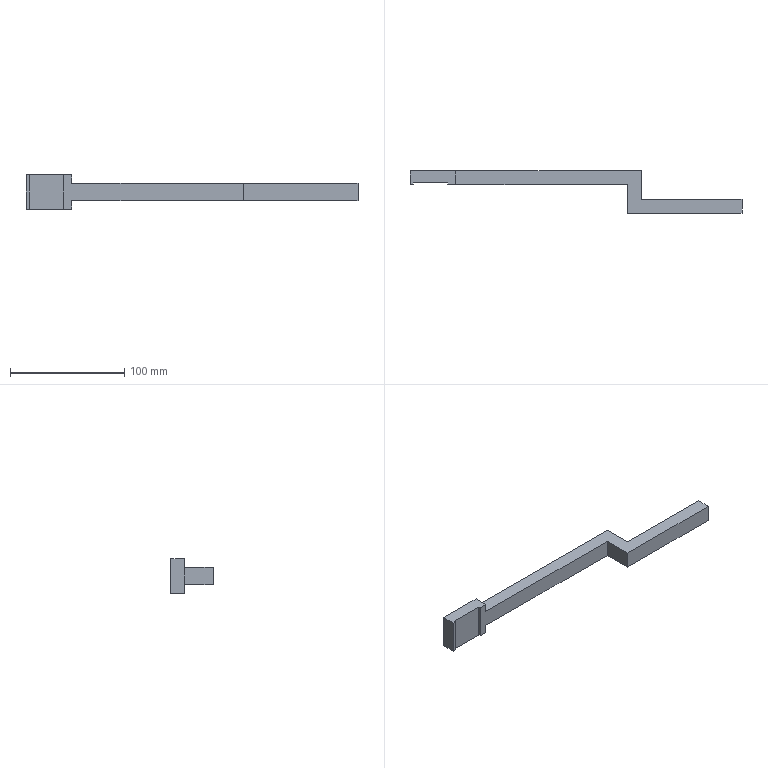Part | SolidWorks | features ICE 2, Extrusion 1 | 1 solid | 18 faces | box 290 x 37 x 30 mm | volume 62550 mm3 | plane 18
STEP:
#1=CARTESIAN_POINT('',(-37.,-12.,-15.));
#2=VERTEX_POINT('',#1);
#3=CARTESIAN_POINT('',(-37.,-12.,15.));
#4=VERTEX_POINT('',#3);
#5=CARTESIAN_POINT('',(-37.,-12.,-15.));
#6=DIRECTION('',(0.,0.,1.));
#7=VECTOR('',#6,1000.);
#8=LINE('',#5,#7);
#9=EDGE_CURVE('',#2,#4,#8,.T.);
#10=ORIENTED_EDGE('',*,*,#9,.T.);
#11=CARTESIAN_POINT('',(-40.,-12.,15.));
#12=VERTEX_POINT('',#11);
#13=CARTESIAN_POINT('',(0.,-12.,15.));
#14=DIRECTION('',(-1.,0.,0.));
#15=VECTOR('',#14,1000.);
#16=LINE('',#13,#15);
#17=EDGE_CURVE('',#4,#12,#16,.T.);
#18=ORIENTED_EDGE('',*,*,#17,.T.);
#19=CARTESIAN_POINT('',(-40.,-12.,-15.));
#20=VERTEX_POINT('',#19);
#21=CARTESIAN_POINT('',(-40.,-12.,15.));
#22=DIRECTION('',(0.,0.,-1.));
#23=VECTOR('',#22,1000.);
#24=LINE('',#21,#23);
#25=EDGE_CURVE('',#12,#20,#24,.T.);
#26=ORIENTED_EDGE('',*,*,#25,.T.);
#27=CARTESIAN_POINT('',(0.,-12.,-15.));
#28=DIRECTION('',(1.,0.,0.));
#29=VECTOR('',#28,1000.);
#30=LINE('',#27,#29);
#31=EDGE_CURVE('',#20,#2,#30,.T.);
#32=ORIENTED_EDGE('',*,*,#31,.T.);
#33=EDGE_LOOP('',(#10,#18,#26,#32));
#34=FACE_OUTER_BOUND('',#33,.T.);
#35=CARTESIAN_POINT('',(150.,-12.,7.5));
#36=DIRECTION('',(0.,1.,0.));
#37=DIRECTION('',(-1.,0.,0.));
#38=AXIS2_PLACEMENT_3D('',#35,#36,#37);
#39=PLANE('',#38);
#40=ADVANCED_FACE('',(#34),#39,.F.);
#41=CARTESIAN_POINT('',(-7.,-12.,15.));
#42=VERTEX_POINT('',#41);
#43=CARTESIAN_POINT('',(-7.,-12.,-15.));
#44=VERTEX_POINT('',#43);
#45=CARTESIAN_POINT('',(-7.,-12.,-15.));
#46=DIRECTION('',(0.,0.,-1.));
#47=VECTOR('',#46,1000.);
#48=LINE('',#45,#47);
#49=EDGE_CURVE('',#42,#44,#48,.T.);
#50=ORIENTED_EDGE('',*,*,#49,.T.);
#51=CARTESIAN_POINT('',(0.,-12.,-15.));
#52=VERTEX_POINT('',#51);
#53=CARTESIAN_POINT('',(0.,-12.,-15.));
#54=DIRECTION('',(1.,0.,0.));
#55=VECTOR('',#54,1000.);
#56=LINE('',#53,#55);
#57=EDGE_CURVE('',#44,#52,#56,.T.);
#58=ORIENTED_EDGE('',*,*,#57,.T.);
#59=CARTESIAN_POINT('',(0.,-12.,-7.5));
#60=VERTEX_POINT('',#59);
#61=CARTESIAN_POINT('',(0.,-12.,15.));
#62=DIRECTION('',(0.,0.,1.));
#63=VECTOR('',#62,1000.);
#64=LINE('',#61,#63);
#65=EDGE_CURVE('',#52,#60,#64,.T.);
#66=ORIENTED_EDGE('',*,*,#65,.T.);
#67=CARTESIAN_POINT('',(150.,-12.,-7.5));
#68=VERTEX_POINT('',#67);
#69=CARTESIAN_POINT('',(150.,-12.,-7.5));
#70=DIRECTION('',(1.,0.,0.));
#71=VECTOR('',#70,1000.);
#72=LINE('',#69,#71);
#73=EDGE_CURVE('',#60,#68,#72,.T.);
#74=ORIENTED_EDGE('',*,*,#73,.T.);
#75=CARTESIAN_POINT('',(150.,-12.,7.5));
#76=VERTEX_POINT('',#75);
#77=CARTESIAN_POINT('',(150.,-12.,7.5));
#78=DIRECTION('',(0.,0.,-1.));
#79=VECTOR('',#78,1000.);
#80=LINE('',#77,#79);
#81=EDGE_CURVE('',#76,#68,#80,.T.);
#82=ORIENTED_EDGE('',*,*,#81,.F.);
#83=CARTESIAN_POINT('',(0.,-12.,7.5));
#84=VERTEX_POINT('',#83);
#85=CARTESIAN_POINT('',(150.,-12.,7.5));
#86=DIRECTION('',(1.,0.,0.));
#87=VECTOR('',#86,1000.);
#88=LINE('',#85,#87);
#89=EDGE_CURVE('',#84,#76,#88,.T.);
#90=ORIENTED_EDGE('',*,*,#89,.F.);
#91=CARTESIAN_POINT('',(0.,-12.,15.));
#92=VERTEX_POINT('',#91);
#93=CARTESIAN_POINT('',(0.,-12.,15.));
#94=DIRECTION('',(0.,0.,1.));
#95=VECTOR('',#94,1000.);
#96=LINE('',#93,#95);
#97=EDGE_CURVE('',#84,#92,#96,.T.);
#98=ORIENTED_EDGE('',*,*,#97,.T.);
#99=CARTESIAN_POINT('',(0.,-12.,15.));
#100=DIRECTION('',(-1.,0.,0.));
#101=VECTOR('',#100,1000.);
#102=LINE('',#99,#101);
#103=EDGE_CURVE('',#92,#42,#102,.T.);
#104=ORIENTED_EDGE('',*,*,#103,.T.);
#105=EDGE_LOOP('',(#50,#58,#66,#74,#82,#90,#98,#104));
#106=FACE_OUTER_BOUND('',#105,.T.);
#107=CARTESIAN_POINT('',(150.,-12.,7.5));
#108=DIRECTION('',(0.,1.,0.));
#109=DIRECTION('',(-1.,0.,0.));
#110=AXIS2_PLACEMENT_3D('',#107,#108,#109);
#111=PLANE('',#110);
#112=ADVANCED_FACE('',(#106),#111,.F.);
#113=CARTESIAN_POINT('',(-7.,-10.5,-15.));
#114=VERTEX_POINT('',#113);
#115=CARTESIAN_POINT('',(-37.,-10.5,-15.));
#116=VERTEX_POINT('',#115);
#117=CARTESIAN_POINT('',(-37.,-10.5,-15.));
#118=DIRECTION('',(-1.,0.,0.));
#119=VECTOR('',#118,1000.);
#120=LINE('',#117,#119);
#121=EDGE_CURVE('',#114,#116,#120,.T.);
#122=ORIENTED_EDGE('',*,*,#121,.T.);
#123=CARTESIAN_POINT('',(-37.,-10.5,-15.));
#124=DIRECTION('',(0.,-1.,0.));
#125=VECTOR('',#124,1000.);
#126=LINE('',#123,#125);
#127=EDGE_CURVE('',#116,#2,#126,.T.);
#128=ORIENTED_EDGE('',*,*,#127,.T.);
#129=ORIENTED_EDGE('',*,*,#31,.F.);
#130=CARTESIAN_POINT('',(-40.,0.,-15.));
#131=VERTEX_POINT('',#130);
#132=CARTESIAN_POINT('',(-40.,-62.,-15.));
#133=DIRECTION('',(0.,1.,0.));
#134=VECTOR('',#133,1000.);
#135=LINE('',#132,#134);
#136=EDGE_CURVE('',#20,#131,#135,.T.);
#137=ORIENTED_EDGE('',*,*,#136,.T.);
#138=CARTESIAN_POINT('',(0.,0.,-15.));
#139=VERTEX_POINT('',#138);
#140=CARTESIAN_POINT('',(0.,0.,-15.));
#141=DIRECTION('',(-1.,0.,0.));
#142=VECTOR('',#141,1000.);
#143=LINE('',#140,#142);
#144=EDGE_CURVE('',#139,#131,#143,.T.);
#145=ORIENTED_EDGE('',*,*,#144,.F.);
#146=CARTESIAN_POINT('',(0.,-62.,-15.));
#147=DIRECTION('',(0.,1.,0.));
#148=VECTOR('',#147,1000.);
#149=LINE('',#146,#148);
#150=EDGE_CURVE('',#52,#139,#149,.T.);
#151=ORIENTED_EDGE('',*,*,#150,.F.);
#152=ORIENTED_EDGE('',*,*,#57,.F.);
#153=CARTESIAN_POINT('',(-7.,-10.5,-15.));
#154=DIRECTION('',(0.,-1.,0.));
#155=VECTOR('',#154,1000.);
#156=LINE('',#153,#155);
#157=EDGE_CURVE('',#114,#44,#156,.T.);
#158=ORIENTED_EDGE('',*,*,#157,.F.);
#159=EDGE_LOOP('',(#122,#128,#129,#137,#145,#151,#152,#158));
#160=FACE_OUTER_BOUND('',#159,.T.);
#161=CARTESIAN_POINT('',(0.,-62.,-15.));
#162=DIRECTION('',(0.,0.,-1.));
#163=DIRECTION('',(-1.,0.,0.));
#164=AXIS2_PLACEMENT_3D('',#161,#162,#163);
#165=PLANE('',#164);
#166=ADVANCED_FACE('',(#160),#165,.T.);
#167=ORIENTED_EDGE('',*,*,#17,.F.);
#168=CARTESIAN_POINT('',(-37.,-10.5,15.));
#169=VERTEX_POINT('',#168);
#170=CARTESIAN_POINT('',(-37.,-10.5,15.));
#171=DIRECTION('',(0.,-1.,0.));
#172=VECTOR('',#171,1000.);
#173=LINE('',#170,#172);
#174=EDGE_CURVE('',#169,#4,#173,.T.);
#175=ORIENTED_EDGE('',*,*,#174,.F.);
#176=CARTESIAN_POINT('',(-7.,-10.5,15.));
#177=VERTEX_POINT('',#176);
#178=CARTESIAN_POINT('',(-37.,-10.5,15.));
#179=DIRECTION('',(1.,0.,0.));
#180=VECTOR('',#179,1000.);
#181=LINE('',#178,#180);
#182=EDGE_CURVE('',#169,#177,#181,.T.);
#183=ORIENTED_EDGE('',*,*,#182,.T.);
#184=CARTESIAN_POINT('',(-7.,-10.5,15.));
#185=DIRECTION('',(0.,-1.,0.));
#186=VECTOR('',#185,1000.);
#187=LINE('',#184,#186);
#188=EDGE_CURVE('',#177,#42,#187,.T.);
#189=ORIENTED_EDGE('',*,*,#188,.T.);
#190=ORIENTED_EDGE('',*,*,#103,.F.);
#191=CARTESIAN_POINT('',(0.,0.,15.));
#192=VERTEX_POINT('',#191);
#193=CARTESIAN_POINT('',(0.,-62.,15.));
#194=DIRECTION('',(0.,1.,0.));
#195=VECTOR('',#194,1000.);
#196=LINE('',#193,#195);
#197=EDGE_CURVE('',#92,#192,#196,.T.);
#198=ORIENTED_EDGE('',*,*,#197,.T.);
#199=CARTESIAN_POINT('',(-40.,0.,15.));
#200=VERTEX_POINT('',#199);
#201=CARTESIAN_POINT('',(0.,0.,15.));
#202=DIRECTION('',(1.,0.,0.));
#203=VECTOR('',#202,1000.);
#204=LINE('',#201,#203);
#205=EDGE_CURVE('',#200,#192,#204,.T.);
#206=ORIENTED_EDGE('',*,*,#205,.F.);
#207=CARTESIAN_POINT('',(-40.,-62.,15.));
#208=DIRECTION('',(0.,1.,0.));
#209=VECTOR('',#208,1000.);
#210=LINE('',#207,#209);
#211=EDGE_CURVE('',#12,#200,#210,.T.);
#212=ORIENTED_EDGE('',*,*,#211,.F.);
#213=EDGE_LOOP('',(#167,#175,#183,#189,#190,#198,#206,#212));
#214=FACE_OUTER_BOUND('',#213,.T.);
#215=CARTESIAN_POINT('',(0.,-62.,15.));
#216=DIRECTION('',(0.,0.,1.));
#217=DIRECTION('',(1.,0.,0.));
#218=AXIS2_PLACEMENT_3D('',#215,#216,#217);
#219=PLANE('',#218);
#220=ADVANCED_FACE('',(#214),#219,.T.);
#221=CARTESIAN_POINT('',(150.,-37.,-7.5));
#222=VERTEX_POINT('',#221);
#223=CARTESIAN_POINT('',(150.,-37.,-7.5));
#224=DIRECTION('',(0.,-1.,0.));
#225=VECTOR('',#224,1000.);
#226=LINE('',#223,#225);
#227=EDGE_CURVE('',#68,#222,#226,.T.);
#228=ORIENTED_EDGE('',*,*,#227,.T.);
#229=CARTESIAN_POINT('',(150.,-37.,7.5));
#230=VERTEX_POINT('',#229);
#231=CARTESIAN_POINT('',(150.,-37.,7.5));
#232=DIRECTION('',(0.,0.,-1.));
#233=VECTOR('',#232,1000.);
#234=LINE('',#231,#233);
#235=EDGE_CURVE('',#230,#222,#234,.T.);
#236=ORIENTED_EDGE('',*,*,#235,.F.);
#237=CARTESIAN_POINT('',(150.,-37.,7.5));
#238=DIRECTION('',(0.,-1.,0.));
#239=VECTOR('',#238,1000.);
#240=LINE('',#237,#239);
#241=EDGE_CURVE('',#76,#230,#240,.T.);
#242=ORIENTED_EDGE('',*,*,#241,.F.);
#243=ORIENTED_EDGE('',*,*,#81,.T.);
#244=EDGE_LOOP('',(#228,#236,#242,#243));
#245=FACE_OUTER_BOUND('',#244,.T.);
#246=CARTESIAN_POINT('',(150.,-37.,7.5));
#247=DIRECTION('',(1.,0.,0.));
#248=DIRECTION('',(0.,0.,-1.));
#249=AXIS2_PLACEMENT_3D('',#246,#247,#248);
#250=PLANE('',#249);
#251=ADVANCED_FACE('',(#245),#250,.F.);
#252=CARTESIAN_POINT('',(250.,-37.,-7.5));
#253=VERTEX_POINT('',#252);
#254=CARTESIAN_POINT('',(250.,-37.,-7.5));
#255=DIRECTION('',(1.,0.,0.));
#256=VECTOR('',#255,1000.);
#257=LINE('',#254,#256);
#258=EDGE_CURVE('',#222,#253,#257,.T.);
#259=ORIENTED_EDGE('',*,*,#258,.T.);
#260=CARTESIAN_POINT('',(250.,-37.,7.5));
#261=VERTEX_POINT('',#260);
#262=CARTESIAN_POINT('',(250.,-37.,7.5));
#263=DIRECTION('',(0.,0.,-1.));
#264=VECTOR('',#263,1000.);
#265=LINE('',#262,#264);
#266=EDGE_CURVE('',#261,#253,#265,.T.);
#267=ORIENTED_EDGE('',*,*,#266,.F.);
#268=CARTESIAN_POINT('',(250.,-37.,7.5));
#269=DIRECTION('',(1.,0.,0.));
#270=VECTOR('',#269,1000.);
#271=LINE('',#268,#270);
#272=EDGE_CURVE('',#230,#261,#271,.T.);
#273=ORIENTED_EDGE('',*,*,#272,.F.);
#274=ORIENTED_EDGE('',*,*,#235,.T.);
#275=EDGE_LOOP('',(#259,#267,#273,#274));
#276=FACE_OUTER_BOUND('',#275,.T.);
#277=CARTESIAN_POINT('',(250.,-37.,7.5));
#278=DIRECTION('',(0.,1.,0.));
#279=DIRECTION('',(-1.,0.,0.));
#280=AXIS2_PLACEMENT_3D('',#277,#278,#279);
#281=PLANE('',#280);
#282=ADVANCED_FACE('',(#276),#281,.F.);
#283=CARTESIAN_POINT('',(250.,-25.,-7.5));
#284=VERTEX_POINT('',#283);
#285=CARTESIAN_POINT('',(250.,-25.,-7.5));
#286=DIRECTION('',(0.,1.,0.));
#287=VECTOR('',#286,1000.);
#288=LINE('',#285,#287);
#289=EDGE_CURVE('',#253,#284,#288,.T.);
#290=ORIENTED_EDGE('',*,*,#289,.T.);
#291=CARTESIAN_POINT('',(250.,-25.,7.5));
#292=VERTEX_POINT('',#291);
#293=CARTESIAN_POINT('',(250.,-25.,7.5));
#294=DIRECTION('',(0.,0.,-1.));
#295=VECTOR('',#294,1000.);
#296=LINE('',#293,#295);
#297=EDGE_CURVE('',#292,#284,#296,.T.);
#298=ORIENTED_EDGE('',*,*,#297,.F.);
#299=CARTESIAN_POINT('',(250.,-25.,7.5));
#300=DIRECTION('',(0.,1.,0.));
#301=VECTOR('',#300,1000.);
#302=LINE('',#299,#301);
#303=EDGE_CURVE('',#261,#292,#302,.T.);
#304=ORIENTED_EDGE('',*,*,#303,.F.);
#305=ORIENTED_EDGE('',*,*,#266,.T.);
#306=EDGE_LOOP('',(#290,#298,#304,#305));
#307=FACE_OUTER_BOUND('',#306,.T.);
#308=CARTESIAN_POINT('',(250.,-25.,7.5));
#309=DIRECTION('',(-1.,0.,0.));
#310=DIRECTION('',(0.,0.,1.));
#311=AXIS2_PLACEMENT_3D('',#308,#309,#310);
#312=PLANE('',#311);
#313=ADVANCED_FACE('',(#307),#312,.F.);
#314=CARTESIAN_POINT('',(162.,-25.,-7.5));
#315=VERTEX_POINT('',#314);
#316=CARTESIAN_POINT('',(162.,-25.,-7.5));
#317=DIRECTION('',(-1.,0.,0.));
#318=VECTOR('',#317,1000.);
#319=LINE('',#316,#318);
#320=EDGE_CURVE('',#284,#315,#319,.T.);
#321=ORIENTED_EDGE('',*,*,#320,.T.);
#322=CARTESIAN_POINT('',(162.,-25.,7.5));
#323=VERTEX_POINT('',#322);
#324=CARTESIAN_POINT('',(162.,-25.,7.5));
#325=DIRECTION('',(0.,0.,-1.));
#326=VECTOR('',#325,1000.);
#327=LINE('',#324,#326);
#328=EDGE_CURVE('',#323,#315,#327,.T.);
#329=ORIENTED_EDGE('',*,*,#328,.F.);
#330=CARTESIAN_POINT('',(162.,-25.,7.5));
#331=DIRECTION('',(-1.,0.,0.));
#332=VECTOR('',#331,1000.);
#333=LINE('',#330,#332);
#334=EDGE_CURVE('',#292,#323,#333,.T.);
#335=ORIENTED_EDGE('',*,*,#334,.F.);
#336=ORIENTED_EDGE('',*,*,#297,.T.);
#337=EDGE_LOOP('',(#321,#329,#335,#336));
#338=FACE_OUTER_BOUND('',#337,.T.);
#339=CARTESIAN_POINT('',(162.,-25.,7.5));
#340=DIRECTION('',(0.,-1.,0.));
#341=DIRECTION('',(0.,0.,-1.));
#342=AXIS2_PLACEMENT_3D('',#339,#340,#341);
#343=PLANE('',#342);
#344=ADVANCED_FACE('',(#338),#343,.F.);
#345=CARTESIAN_POINT('',(162.,0.,-7.5));
#346=VERTEX_POINT('',#345);
#347=CARTESIAN_POINT('',(162.,0.,-7.5));
#348=DIRECTION('',(0.,1.,0.));
#349=VECTOR('',#348,1000.);
#350=LINE('',#347,#349);
#351=EDGE_CURVE('',#315,#346,#350,.T.);
#352=ORIENTED_EDGE('',*,*,#351,.T.);
#353=CARTESIAN_POINT('',(162.,0.,7.5));
#354=VERTEX_POINT('',#353);
#355=CARTESIAN_POINT('',(162.,0.,7.5));
#356=DIRECTION('',(0.,0.,-1.));
#357=VECTOR('',#356,1000.);
#358=LINE('',#355,#357);
#359=EDGE_CURVE('',#354,#346,#358,.T.);
#360=ORIENTED_EDGE('',*,*,#359,.F.);
#361=CARTESIAN_POINT('',(162.,0.,7.5));
#362=DIRECTION('',(0.,1.,0.));
#363=VECTOR('',#362,1000.);
#364=LINE('',#361,#363);
#365=EDGE_CURVE('',#323,#354,#364,.T.);
#366=ORIENTED_EDGE('',*,*,#365,.F.);
#367=ORIENTED_EDGE('',*,*,#328,.T.);
#368=EDGE_LOOP('',(#352,#360,#366,#367));
#369=FACE_OUTER_BOUND('',#368,.T.);
#370=CARTESIAN_POINT('',(162.,0.,7.5));
#371=DIRECTION('',(-1.,0.,0.));
#372=DIRECTION('',(0.,0.,1.));
#373=AXIS2_PLACEMENT_3D('',#370,#371,#372);
#374=PLANE('',#373);
#375=ADVANCED_FACE('',(#369),#374,.F.);
#376=CARTESIAN_POINT('',(0.,0.,-7.5));
#377=VERTEX_POINT('',#376);
#378=CARTESIAN_POINT('',(0.,0.,-7.5));
#379=DIRECTION('',(-1.,0.,0.));
#380=VECTOR('',#379,1000.);
#381=LINE('',#378,#380);
#382=EDGE_CURVE('',#346,#377,#381,.T.);
#383=ORIENTED_EDGE('',*,*,#382,.T.);
#384=CARTESIAN_POINT('',(0.,0.,15.));
#385=DIRECTION('',(0.,0.,-1.));
#386=VECTOR('',#385,1000.);
#387=LINE('',#384,#386);
#388=EDGE_CURVE('',#377,#139,#387,.T.);
#389=ORIENTED_EDGE('',*,*,#388,.T.);
#390=ORIENTED_EDGE('',*,*,#144,.T.);
#391=CARTESIAN_POINT('',(-40.,0.,15.));
#392=DIRECTION('',(0.,0.,1.));
#393=VECTOR('',#392,1000.);
#394=LINE('',#391,#393);
#395=EDGE_CURVE('',#131,#200,#394,.T.);
#396=ORIENTED_EDGE('',*,*,#395,.T.);
#397=ORIENTED_EDGE('',*,*,#205,.T.);
#398=CARTESIAN_POINT('',(0.,0.,7.5));
#399=VERTEX_POINT('',#398);
#400=CARTESIAN_POINT('',(0.,0.,15.));
#401=DIRECTION('',(0.,0.,-1.));
#402=VECTOR('',#401,1000.);
#403=LINE('',#400,#402);
#404=EDGE_CURVE('',#192,#399,#403,.T.);
#405=ORIENTED_EDGE('',*,*,#404,.T.);
#406=CARTESIAN_POINT('',(0.,0.,7.5));
#407=DIRECTION('',(-1.,0.,0.));
#408=VECTOR('',#407,1000.);
#409=LINE('',#406,#408);
#410=EDGE_CURVE('',#354,#399,#409,.T.);
#411=ORIENTED_EDGE('',*,*,#410,.F.);
#412=ORIENTED_EDGE('',*,*,#359,.T.);
#413=EDGE_LOOP('',(#383,#389,#390,#396,#397,#405,#411,#412));
#414=FACE_OUTER_BOUND('',#413,.T.);
#415=CARTESIAN_POINT('',(0.,0.,7.5));
#416=DIRECTION('',(0.,-1.,0.));
#417=DIRECTION('',(0.,0.,-1.));
#418=AXIS2_PLACEMENT_3D('',#415,#416,#417);
#419=PLANE('',#418);
#420=ADVANCED_FACE('',(#414),#419,.F.);
#421=CARTESIAN_POINT('',(0.,-12.,7.5));
#422=DIRECTION('',(0.,-1.,0.));
#423=VECTOR('',#422,1000.);
#424=LINE('',#421,#423);
#425=EDGE_CURVE('',#399,#84,#424,.T.);
#426=ORIENTED_EDGE('',*,*,#425,.T.);
#427=ORIENTED_EDGE('',*,*,#89,.T.);
#428=ORIENTED_EDGE('',*,*,#241,.T.);
#429=ORIENTED_EDGE('',*,*,#272,.T.);
#430=ORIENTED_EDGE('',*,*,#303,.T.);
#431=ORIENTED_EDGE('',*,*,#334,.T.);
#432=ORIENTED_EDGE('',*,*,#365,.T.);
#433=ORIENTED_EDGE('',*,*,#410,.T.);
#434=EDGE_LOOP('',(#426,#427,#428,#429,#430,#431,#432,#433));
#435=FACE_OUTER_BOUND('',#434,.T.);
#436=CARTESIAN_POINT('',(0.,0.,7.5));
#437=DIRECTION('',(0.,0.,-1.));
#438=DIRECTION('',(-1.,0.,0.));
#439=AXIS2_PLACEMENT_3D('',#436,#437,#438);
#440=PLANE('',#439);
#441=ADVANCED_FACE('',(#435),#440,.F.);
#442=CARTESIAN_POINT('',(0.,-12.,-7.5));
#443=DIRECTION('',(0.,-1.,0.));
#444=VECTOR('',#443,1000.);
#445=LINE('',#442,#444);
#446=EDGE_CURVE('',#377,#60,#445,.T.);
#447=ORIENTED_EDGE('',*,*,#446,.F.);
#448=ORIENTED_EDGE('',*,*,#382,.F.);
#449=ORIENTED_EDGE('',*,*,#351,.F.);
#450=ORIENTED_EDGE('',*,*,#320,.F.);
#451=ORIENTED_EDGE('',*,*,#289,.F.);
#452=ORIENTED_EDGE('',*,*,#258,.F.);
#453=ORIENTED_EDGE('',*,*,#227,.F.);
#454=ORIENTED_EDGE('',*,*,#73,.F.);
#455=EDGE_LOOP('',(#447,#448,#449,#450,#451,#452,#453,#454));
#456=FACE_OUTER_BOUND('',#455,.T.);
#457=CARTESIAN_POINT('',(0.,0.,-7.5));
#458=DIRECTION('',(0.,0.,-1.));
#459=DIRECTION('',(-1.,0.,0.));
#460=AXIS2_PLACEMENT_3D('',#457,#458,#459);
#461=PLANE('',#460);
#462=ADVANCED_FACE('',(#456),#461,.T.);
#463=ORIENTED_EDGE('',*,*,#425,.F.);
#464=ORIENTED_EDGE('',*,*,#404,.F.);
#465=ORIENTED_EDGE('',*,*,#197,.F.);
#466=ORIENTED_EDGE('',*,*,#97,.F.);
#467=EDGE_LOOP('',(#463,#464,#465,#466));
#468=FACE_OUTER_BOUND('',#467,.T.);
#469=CARTESIAN_POINT('',(0.,-62.,15.));
#470=DIRECTION('',(1.,0.,0.));
#471=DIRECTION('',(0.,0.,-1.));
#472=AXIS2_PLACEMENT_3D('',#469,#470,#471);
#473=PLANE('',#472);
#474=ADVANCED_FACE('',(#468),#473,.T.);
#475=ORIENTED_EDGE('',*,*,#25,.F.);
#476=ORIENTED_EDGE('',*,*,#211,.T.);
#477=ORIENTED_EDGE('',*,*,#395,.F.);
#478=ORIENTED_EDGE('',*,*,#136,.F.);
#479=EDGE_LOOP('',(#475,#476,#477,#478));
#480=FACE_OUTER_BOUND('',#479,.T.);
#481=CARTESIAN_POINT('',(-40.,-62.,15.));
#482=DIRECTION('',(-1.,0.,0.));
#483=DIRECTION('',(0.,0.,1.));
#484=AXIS2_PLACEMENT_3D('',#481,#482,#483);
#485=PLANE('',#484);
#486=ADVANCED_FACE('',(#480),#485,.T.);
#487=ORIENTED_EDGE('',*,*,#388,.F.);
#488=ORIENTED_EDGE('',*,*,#446,.T.);
#489=ORIENTED_EDGE('',*,*,#65,.F.);
#490=ORIENTED_EDGE('',*,*,#150,.T.);
#491=EDGE_LOOP('',(#487,#488,#489,#490));
#492=FACE_OUTER_BOUND('',#491,.T.);
#493=CARTESIAN_POINT('',(0.,-62.,15.));
#494=DIRECTION('',(1.,0.,0.));
#495=DIRECTION('',(0.,0.,-1.));
#496=AXIS2_PLACEMENT_3D('',#493,#494,#495);
#497=PLANE('',#496);
#498=ADVANCED_FACE('',(#492),#497,.T.);
#499=ORIENTED_EDGE('',*,*,#9,.F.);
#500=ORIENTED_EDGE('',*,*,#127,.F.);
#501=CARTESIAN_POINT('',(-37.,-10.5,-15.));
#502=DIRECTION('',(0.,0.,1.));
#503=VECTOR('',#502,1000.);
#504=LINE('',#501,#503);
#505=EDGE_CURVE('',#116,#169,#504,.T.);
#506=ORIENTED_EDGE('',*,*,#505,.T.);
#507=ORIENTED_EDGE('',*,*,#174,.T.);
#508=EDGE_LOOP('',(#499,#500,#506,#507));
#509=FACE_OUTER_BOUND('',#508,.T.);
#510=CARTESIAN_POINT('',(-37.,-10.5,-15.));
#511=DIRECTION('',(1.,0.,0.));
#512=DIRECTION('',(0.,0.,-1.));
#513=AXIS2_PLACEMENT_3D('',#510,#511,#512);
#514=PLANE('',#513);
#515=ADVANCED_FACE('',(#509),#514,.T.);
#516=ORIENTED_EDGE('',*,*,#49,.F.);
#517=ORIENTED_EDGE('',*,*,#188,.F.);
#518=CARTESIAN_POINT('',(-7.,-10.5,-15.));
#519=DIRECTION('',(0.,0.,-1.));
#520=VECTOR('',#519,1000.);
#521=LINE('',#518,#520);
#522=EDGE_CURVE('',#177,#114,#521,.T.);
#523=ORIENTED_EDGE('',*,*,#522,.T.);
#524=ORIENTED_EDGE('',*,*,#157,.T.);
#525=EDGE_LOOP('',(#516,#517,#523,#524));
#526=FACE_OUTER_BOUND('',#525,.T.);
#527=CARTESIAN_POINT('',(-7.,-10.5,-15.));
#528=DIRECTION('',(-1.,0.,0.));
#529=DIRECTION('',(0.,-1.,0.));
#530=AXIS2_PLACEMENT_3D('',#527,#528,#529);
#531=PLANE('',#530);
#532=ADVANCED_FACE('',(#526),#531,.T.);
#533=ORIENTED_EDGE('',*,*,#505,.F.);
#534=ORIENTED_EDGE('',*,*,#121,.F.);
#535=ORIENTED_EDGE('',*,*,#522,.F.);
#536=ORIENTED_EDGE('',*,*,#182,.F.);
#537=EDGE_LOOP('',(#533,#534,#535,#536));
#538=FACE_OUTER_BOUND('',#537,.T.);
#539=CARTESIAN_POINT('',(0.,-10.5,0.));
#540=DIRECTION('',(0.,1.,0.));
#541=DIRECTION('',(-1.,0.,0.));
#542=AXIS2_PLACEMENT_3D('',#539,#540,#541);
#543=PLANE('',#542);
#544=ADVANCED_FACE('',(#538),#543,.F.);
#545=CLOSED_SHELL('',(#40,#112,#166,#220,#251,#282,#313,#344,#375,#420,#441,#462,#474,#486,#498,#515,#532,#544));
#546=MANIFOLD_SOLID_BREP('',#545);
#547=CARTESIAN_POINT('',(0.,0.,0.));
#548=DIRECTION('',(0.,0.,1.));
#549=DIRECTION('',(1.,0.,0.));
#550=AXIS2_PLACEMENT_3D('',#547,#548,#549);
#551=(LENGTH_UNIT()NAMED_UNIT(*)SI_UNIT(.MILLI.,.METRE.));
#552=UNCERTAINTY_MEASURE_WITH_UNIT(LENGTH_MEASURE(0.00001),#551,'','');
#553=(NAMED_UNIT(*)PLANE_ANGLE_UNIT()SI_UNIT($,.RADIAN.));
#554=(NAMED_UNIT(*)SI_UNIT($,.STERADIAN.)SOLID_ANGLE_UNIT());
#555=(GEOMETRIC_REPRESENTATION_CONTEXT(3)GLOBAL_UNCERTAINTY_ASSIGNED_CONTEXT((#552))GLOBAL_UNIT_ASSIGNED_CONTEXT((#551,#553,#554))REPRESENTATION_CONTEXT('',''));
#556=ADVANCED_BREP_SHAPE_REPRESENTATION('',(#546,#550),#555);